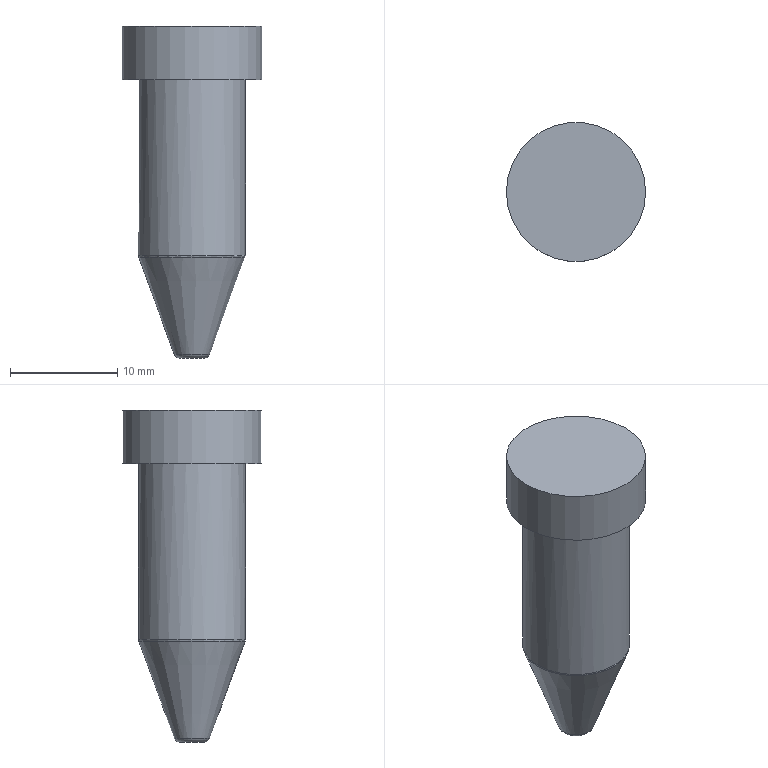Part | STEP file | gslz 2016.10.28-10_id3046_x_t | 1 solid | 8 faces | box 13 x 13 x 31 mm | volume 2308 mm3 | plane 3 | cylinder 2 | torus 2 | cone 1 | commonest cylinder face diameters 10 x1 13 x1
STEP:
#1=CARTESIAN_POINT('',(0.,0.,0.));
#2=DIRECTION('',(0.,0.,1.));
#3=DIRECTION('',(1.,0.,0.));
#4=AXIS2_PLACEMENT_3D('',#1,#2,#3);
#5=CARTESIAN_POINT('',(-528.808,157.,-11.));
#6=VERTEX_POINT('',#5);
#7=CARTESIAN_POINT('',(-531.192,157.,-11.));
#8=VERTEX_POINT('',#7);
#9=CARTESIAN_POINT('',(-530.,157.,-11.));
#10=DIRECTION('',(0.,0.,-1.));
#11=DIRECTION('',(1.,0.,0.));
#12=AXIS2_PLACEMENT_3D('',#9,#10,#11);
#13=CIRCLE('',#12,1.192);
#14=CARTESIAN_POINT('',(-530.,157.,-11.));
#15=DIRECTION('',(0.,0.,1.));
#16=DIRECTION('',(-1.,0.,0.));
#17=AXIS2_PLACEMENT_3D('',#14,#15,#16);
#18=PLANE('',#17);
#19=CARTESIAN_POINT('',(-1.192,0.));
#20=CARTESIAN_POINT('',(-1.192,2.065));
#21=CARTESIAN_POINT('',(0.5961,1.032));
#22=CARTESIAN_POINT('',(2.384,0.));
#23=CARTESIAN_POINT('',(0.5961,-1.032));
#24=CARTESIAN_POINT('',(-1.192,-2.065));
#25=CARTESIAN_POINT('',(-1.192,0.));
#26=(BOUNDED_CURVE()B_SPLINE_CURVE(2,(#19,#20,#21,#22,#23,#24,#25),.UNSPECIFIED.,.T.,.F.)B_SPLINE_CURVE_WITH_KNOTS((1,2,2,2,2,1),(-2.094,0.,2.094,4.189,6.283,8.378),.UNSPECIFIED.)CURVE()GEOMETRIC_REPRESENTATION_ITEM()RATIONAL_B_SPLINE_CURVE((1.,0.5,1.,0.5,1.,0.5,1.))REPRESENTATION_ITEM(''));
#27=(GEOMETRIC_REPRESENTATION_CONTEXT(2)PARAMETRIC_REPRESENTATION_CONTEXT()REPRESENTATION_CONTEXT('',''));
#28=DEFINITIONAL_REPRESENTATION('',(#26),#27);
#29=PCURVE('',#18,#28);
#30=CARTESIAN_POINT('',(-530.,157.,-10.5));
#31=DIRECTION('',(0.,0.,1.));
#32=DIRECTION('',(-1.,0.,0.));
#33=AXIS2_PLACEMENT_3D('',#30,#31,#32);
#34=TOROIDAL_SURFACE('',#33,1.192,0.5);
#35=CARTESIAN_POINT('',(3.142,4.712));
#36=DIRECTION('',(-1.,0.));
#37=VECTOR('',#36,1.);
#38=LINE('',#35,#37);
#39=(GEOMETRIC_REPRESENTATION_CONTEXT(2)PARAMETRIC_REPRESENTATION_CONTEXT()REPRESENTATION_CONTEXT('',''));
#40=DEFINITIONAL_REPRESENTATION('',(#38),#39);
#41=PCURVE('',#34,#40);
#42=SURFACE_CURVE('',#13,(#29,#41),.PCURVE_S1.);
#43=EDGE_CURVE('',#6,#8,#42,.T.);
#44=ORIENTED_EDGE('',*,*,#43,.T.);
#45=CARTESIAN_POINT('',(-530.,157.,-11.));
#46=DIRECTION('',(0.,0.,-1.));
#47=DIRECTION('',(1.,0.,0.));
#48=AXIS2_PLACEMENT_3D('',#45,#46,#47);
#49=CIRCLE('',#48,1.192);
#50=CARTESIAN_POINT('',(-1.192,0.));
#51=CARTESIAN_POINT('',(-1.192,2.065));
#52=CARTESIAN_POINT('',(0.5961,1.032));
#53=CARTESIAN_POINT('',(2.384,0.));
#54=CARTESIAN_POINT('',(0.5961,-1.032));
#55=CARTESIAN_POINT('',(-1.192,-2.065));
#56=CARTESIAN_POINT('',(-1.192,0.));
#57=(BOUNDED_CURVE()B_SPLINE_CURVE(2,(#50,#51,#52,#53,#54,#55,#56),.UNSPECIFIED.,.T.,.F.)B_SPLINE_CURVE_WITH_KNOTS((1,2,2,2,2,1),(-2.094,0.,2.094,4.189,6.283,8.378),.UNSPECIFIED.)CURVE()GEOMETRIC_REPRESENTATION_ITEM()RATIONAL_B_SPLINE_CURVE((1.,0.5,1.,0.5,1.,0.5,1.))REPRESENTATION_ITEM(''));
#58=(GEOMETRIC_REPRESENTATION_CONTEXT(2)PARAMETRIC_REPRESENTATION_CONTEXT()REPRESENTATION_CONTEXT('',''));
#59=DEFINITIONAL_REPRESENTATION('',(#57),#58);
#60=PCURVE('',#18,#59);
#61=CARTESIAN_POINT('',(9.425,4.712));
#62=DIRECTION('',(-1.,0.));
#63=VECTOR('',#62,1.);
#64=LINE('',#61,#63);
#65=(GEOMETRIC_REPRESENTATION_CONTEXT(2)PARAMETRIC_REPRESENTATION_CONTEXT()REPRESENTATION_CONTEXT('',''));
#66=DEFINITIONAL_REPRESENTATION('',(#64),#65);
#67=PCURVE('',#34,#66);
#68=SURFACE_CURVE('',#49,(#60,#67),.PCURVE_S1.);
#69=EDGE_CURVE('',#8,#6,#68,.T.);
#70=ORIENTED_EDGE('',*,*,#69,.T.);
#71=EDGE_LOOP('',(#44,#70));
#72=FACE_BOUND('',#71,.T.);
#73=ADVANCED_FACE('',(#72),#18,.F.);
#74=CARTESIAN_POINT('',(-525.,157.,-1.412));
#75=VERTEX_POINT('',#74);
#76=CARTESIAN_POINT('',(-535.,157.,-1.412));
#77=VERTEX_POINT('',#76);
#78=CARTESIAN_POINT('',(-530.,157.,-1.412));
#79=DIRECTION('',(0.,0.,1.));
#80=DIRECTION('',(1.,0.,0.));
#81=AXIS2_PLACEMENT_3D('',#78,#79,#80);
#82=CIRCLE('',#81,5.);
#83=CARTESIAN_POINT('',(-530.,157.,11.));
#84=DIRECTION('',(0.,0.,-1.));
#85=DIRECTION('',(1.,0.,0.));
#86=AXIS2_PLACEMENT_3D('',#83,#84,#85);
#87=CYLINDRICAL_SURFACE('',#86,5.);
#88=CARTESIAN_POINT('',(6.283,12.412));
#89=DIRECTION('',(-1.,0.));
#90=VECTOR('',#89,1.);
#91=LINE('',#88,#90);
#92=(GEOMETRIC_REPRESENTATION_CONTEXT(2)PARAMETRIC_REPRESENTATION_CONTEXT()REPRESENTATION_CONTEXT('',''));
#93=DEFINITIONAL_REPRESENTATION('',(#91),#92);
#94=PCURVE('',#87,#93);
#95=CARTESIAN_POINT('',(-530.,157.,-1.412));
#96=DIRECTION('',(0.,0.,1.));
#97=DIRECTION('',(-1.,0.,0.));
#98=AXIS2_PLACEMENT_3D('',#95,#96,#97);
#99=TOROIDAL_SURFACE('',#98,4.5,0.5);
#100=CARTESIAN_POINT('',(3.142,6.283));
#101=DIRECTION('',(1.,0.));
#102=VECTOR('',#101,1.);
#103=LINE('',#100,#102);
#104=(GEOMETRIC_REPRESENTATION_CONTEXT(2)PARAMETRIC_REPRESENTATION_CONTEXT()REPRESENTATION_CONTEXT('',''));
#105=DEFINITIONAL_REPRESENTATION('',(#103),#104);
#106=PCURVE('',#99,#105);
#107=SURFACE_CURVE('',#82,(#94,#106),.PCURVE_S1.);
#108=EDGE_CURVE('',#75,#77,#107,.T.);
#109=ORIENTED_EDGE('',*,*,#108,.T.);
#110=CARTESIAN_POINT('',(-530.,157.,-1.412));
#111=DIRECTION('',(0.,0.,1.));
#112=DIRECTION('',(1.,0.,0.));
#113=AXIS2_PLACEMENT_3D('',#110,#111,#112);
#114=CIRCLE('',#113,5.);
#115=CARTESIAN_POINT('',(6.283,12.412));
#116=DIRECTION('',(-1.,0.));
#117=VECTOR('',#116,1.);
#118=LINE('',#115,#117);
#119=(GEOMETRIC_REPRESENTATION_CONTEXT(2)PARAMETRIC_REPRESENTATION_CONTEXT()REPRESENTATION_CONTEXT('',''));
#120=DEFINITIONAL_REPRESENTATION('',(#118),#119);
#121=PCURVE('',#87,#120);
#122=CARTESIAN_POINT('',(-3.142,6.283));
#123=DIRECTION('',(1.,0.));
#124=VECTOR('',#123,1.);
#125=LINE('',#122,#124);
#126=(GEOMETRIC_REPRESENTATION_CONTEXT(2)PARAMETRIC_REPRESENTATION_CONTEXT()REPRESENTATION_CONTEXT('',''));
#127=DEFINITIONAL_REPRESENTATION('',(#125),#126);
#128=PCURVE('',#99,#127);
#129=SURFACE_CURVE('',#114,(#121,#128),.PCURVE_S1.);
#130=EDGE_CURVE('',#77,#75,#129,.T.);
#131=ORIENTED_EDGE('',*,*,#130,.T.);
#132=CARTESIAN_POINT('',(-525.,157.,15.));
#133=VERTEX_POINT('',#132);
#134=CARTESIAN_POINT('',(-525.,157.,15.));
#135=CARTESIAN_POINT('',(-525.,157.,-1.412));
#136=B_SPLINE_CURVE_WITH_KNOTS('',1,(#134,#135),.UNSPECIFIED.,.F.,.F.,(2,2),(-4.,12.412),.PIECEWISE_BEZIER_KNOTS.);
#137=CARTESIAN_POINT('',(0.,0.));
#138=DIRECTION('',(0.,1.));
#139=VECTOR('',#138,1.);
#140=LINE('',#137,#139);
#141=(GEOMETRIC_REPRESENTATION_CONTEXT(2)PARAMETRIC_REPRESENTATION_CONTEXT()REPRESENTATION_CONTEXT('',''));
#142=DEFINITIONAL_REPRESENTATION('',(#140),#141);
#143=PCURVE('',#87,#142);
#144=CARTESIAN_POINT('',(6.283,0.));
#145=DIRECTION('',(0.,1.));
#146=VECTOR('',#145,1.);
#147=LINE('',#144,#146);
#148=(GEOMETRIC_REPRESENTATION_CONTEXT(2)PARAMETRIC_REPRESENTATION_CONTEXT()REPRESENTATION_CONTEXT('',''));
#149=DEFINITIONAL_REPRESENTATION('',(#147),#148);
#150=PCURVE('',#87,#149);
#151=SEAM_CURVE('',#136,(#143,#150),.PCURVE_S1.);
#152=EDGE_CURVE('',#133,#75,#151,.T.);
#153=ORIENTED_EDGE('',*,*,#152,.F.);
#154=CARTESIAN_POINT('',(-530.,157.,15.));
#155=DIRECTION('',(0.,0.,-1.));
#156=DIRECTION('',(1.,0.,0.));
#157=AXIS2_PLACEMENT_3D('',#154,#155,#156);
#158=CIRCLE('',#157,5.);
#159=CARTESIAN_POINT('',(0.,-4.));
#160=DIRECTION('',(1.,0.));
#161=VECTOR('',#160,1.);
#162=LINE('',#159,#161);
#163=(GEOMETRIC_REPRESENTATION_CONTEXT(2)PARAMETRIC_REPRESENTATION_CONTEXT()REPRESENTATION_CONTEXT('',''));
#164=DEFINITIONAL_REPRESENTATION('',(#162),#163);
#165=PCURVE('',#87,#164);
#166=CARTESIAN_POINT('',(-530.,157.,15.));
#167=DIRECTION('',(0.,0.,-1.));
#168=DIRECTION('',(1.,0.,0.));
#169=AXIS2_PLACEMENT_3D('',#166,#167,#168);
#170=PLANE('',#169);
#171=CARTESIAN_POINT('',(0.,0.));
#172=DIRECTION('',(1.,0.));
#173=AXIS2_PLACEMENT_2D('',#171,#172);
#174=CIRCLE('',#173,5.);
#175=(GEOMETRIC_REPRESENTATION_CONTEXT(2)PARAMETRIC_REPRESENTATION_CONTEXT()REPRESENTATION_CONTEXT('',''));
#176=DEFINITIONAL_REPRESENTATION('',(#174),#175);
#177=PCURVE('',#170,#176);
#178=SURFACE_CURVE('',#158,(#165,#177),.PCURVE_S1.);
#179=EDGE_CURVE('',#133,#133,#178,.T.);
#180=ORIENTED_EDGE('',*,*,#179,.T.);
#181=ORIENTED_EDGE('',*,*,#152,.T.);
#182=EDGE_LOOP('',(#109,#131,#153,#180,#181));
#183=FACE_BOUND('',#182,.T.);
#184=ADVANCED_FACE('',(#183),#87,.T.);
#185=CARTESIAN_POINT('',(-523.5,157.,15.));
#186=VERTEX_POINT('',#185);
#187=CARTESIAN_POINT('',(-530.,157.,15.));
#188=DIRECTION('',(0.,0.,1.));
#189=DIRECTION('',(1.,0.,0.));
#190=AXIS2_PLACEMENT_3D('',#187,#188,#189);
#191=CIRCLE('',#190,6.5);
#192=CARTESIAN_POINT('',(6.5,0.));
#193=CARTESIAN_POINT('',(6.5,-11.258));
#194=CARTESIAN_POINT('',(-3.25,-5.629));
#195=CARTESIAN_POINT('',(-13.,0.));
#196=CARTESIAN_POINT('',(-3.25,5.629));
#197=CARTESIAN_POINT('',(6.5,11.258));
#198=CARTESIAN_POINT('',(6.5,0.));
#199=(BOUNDED_CURVE()B_SPLINE_CURVE(2,(#192,#193,#194,#195,#196,#197,#198),.UNSPECIFIED.,.T.,.F.)B_SPLINE_CURVE_WITH_KNOTS((1,2,2,2,2,1),(-2.094,0.,2.094,4.189,6.283,8.378),.UNSPECIFIED.)CURVE()GEOMETRIC_REPRESENTATION_ITEM()RATIONAL_B_SPLINE_CURVE((1.,0.5,1.,0.5,1.,0.5,1.))REPRESENTATION_ITEM(''));
#200=(GEOMETRIC_REPRESENTATION_CONTEXT(2)PARAMETRIC_REPRESENTATION_CONTEXT()REPRESENTATION_CONTEXT('',''));
#201=DEFINITIONAL_REPRESENTATION('',(#199),#200);
#202=PCURVE('',#170,#201);
#203=CARTESIAN_POINT('',(-530.,157.,20.));
#204=DIRECTION('',(0.,0.,-1.));
#205=DIRECTION('',(1.,0.,0.));
#206=AXIS2_PLACEMENT_3D('',#203,#204,#205);
#207=CYLINDRICAL_SURFACE('',#206,6.5);
#208=CARTESIAN_POINT('',(6.283,5.));
#209=DIRECTION('',(-1.,0.));
#210=VECTOR('',#209,1.);
#211=LINE('',#208,#210);
#212=(GEOMETRIC_REPRESENTATION_CONTEXT(2)PARAMETRIC_REPRESENTATION_CONTEXT()REPRESENTATION_CONTEXT('',''));
#213=DEFINITIONAL_REPRESENTATION('',(#211),#212);
#214=PCURVE('',#207,#213);
#215=SURFACE_CURVE('',#191,(#202,#214),.PCURVE_S1.);
#216=EDGE_CURVE('',#186,#186,#215,.T.);
#217=ORIENTED_EDGE('',*,*,#216,.F.);
#218=EDGE_LOOP('',(#217));
#219=FACE_BOUND('',#218,.T.);
#220=ORIENTED_EDGE('',*,*,#179,.F.);
#221=EDGE_LOOP('',(#220));
#222=FACE_BOUND('',#221,.T.);
#223=ADVANCED_FACE('',(#219,#222),#170,.T.);
#224=CARTESIAN_POINT('',(-536.5,157.,20.));
#225=VERTEX_POINT('',#224);
#226=CARTESIAN_POINT('',(-523.5,157.,20.));
#227=VERTEX_POINT('',#226);
#228=CARTESIAN_POINT('',(-530.,157.,20.));
#229=DIRECTION('',(0.,0.,-1.));
#230=DIRECTION('',(-1.,0.,0.));
#231=AXIS2_PLACEMENT_3D('',#228,#229,#230);
#232=CIRCLE('',#231,6.5);
#233=CARTESIAN_POINT('',(-530.,157.,20.));
#234=DIRECTION('',(0.,0.,1.));
#235=DIRECTION('',(-1.,0.,0.));
#236=AXIS2_PLACEMENT_3D('',#233,#234,#235);
#237=PLANE('',#236);
#238=CARTESIAN_POINT('',(6.5,0.));
#239=CARTESIAN_POINT('',(6.5,-11.258));
#240=CARTESIAN_POINT('',(-3.25,-5.629));
#241=CARTESIAN_POINT('',(-13.,0.));
#242=CARTESIAN_POINT('',(-3.25,5.629));
#243=CARTESIAN_POINT('',(6.5,11.258));
#244=CARTESIAN_POINT('',(6.5,0.));
#245=(BOUNDED_CURVE()B_SPLINE_CURVE(2,(#238,#239,#240,#241,#242,#243,#244),.UNSPECIFIED.,.T.,.F.)B_SPLINE_CURVE_WITH_KNOTS((1,2,2,2,2,1),(-2.094,0.,2.094,4.189,6.283,8.378),.UNSPECIFIED.)CURVE()GEOMETRIC_REPRESENTATION_ITEM()RATIONAL_B_SPLINE_CURVE((1.,0.5,1.,0.5,1.,0.5,1.))REPRESENTATION_ITEM(''));
#246=(GEOMETRIC_REPRESENTATION_CONTEXT(2)PARAMETRIC_REPRESENTATION_CONTEXT()REPRESENTATION_CONTEXT('',''));
#247=DEFINITIONAL_REPRESENTATION('',(#245),#246);
#248=PCURVE('',#237,#247);
#249=CARTESIAN_POINT('',(3.142,0.));
#250=DIRECTION('',(1.,0.));
#251=VECTOR('',#250,1.);
#252=LINE('',#249,#251);
#253=(GEOMETRIC_REPRESENTATION_CONTEXT(2)PARAMETRIC_REPRESENTATION_CONTEXT()REPRESENTATION_CONTEXT('',''));
#254=DEFINITIONAL_REPRESENTATION('',(#252),#253);
#255=PCURVE('',#207,#254);
#256=SURFACE_CURVE('',#232,(#248,#255),.PCURVE_S1.);
#257=EDGE_CURVE('',#225,#227,#256,.T.);
#258=ORIENTED_EDGE('',*,*,#257,.F.);
#259=CARTESIAN_POINT('',(-530.,157.,20.));
#260=DIRECTION('',(0.,0.,-1.));
#261=DIRECTION('',(-1.,0.,0.));
#262=AXIS2_PLACEMENT_3D('',#259,#260,#261);
#263=CIRCLE('',#262,6.5);
#264=CARTESIAN_POINT('',(6.5,0.));
#265=CARTESIAN_POINT('',(6.5,-11.258));
#266=CARTESIAN_POINT('',(-3.25,-5.629));
#267=CARTESIAN_POINT('',(-13.,0.));
#268=CARTESIAN_POINT('',(-3.25,5.629));
#269=CARTESIAN_POINT('',(6.5,11.258));
#270=CARTESIAN_POINT('',(6.5,0.));
#271=(BOUNDED_CURVE()B_SPLINE_CURVE(2,(#264,#265,#266,#267,#268,#269,#270),.UNSPECIFIED.,.T.,.F.)B_SPLINE_CURVE_WITH_KNOTS((1,2,2,2,2,1),(-2.094,0.,2.094,4.189,6.283,8.378),.UNSPECIFIED.)CURVE()GEOMETRIC_REPRESENTATION_ITEM()RATIONAL_B_SPLINE_CURVE((1.,0.5,1.,0.5,1.,0.5,1.))REPRESENTATION_ITEM(''));
#272=(GEOMETRIC_REPRESENTATION_CONTEXT(2)PARAMETRIC_REPRESENTATION_CONTEXT()REPRESENTATION_CONTEXT('',''));
#273=DEFINITIONAL_REPRESENTATION('',(#271),#272);
#274=PCURVE('',#237,#273);
#275=CARTESIAN_POINT('',(-3.142,0.));
#276=DIRECTION('',(1.,0.));
#277=VECTOR('',#276,1.);
#278=LINE('',#275,#277);
#279=(GEOMETRIC_REPRESENTATION_CONTEXT(2)PARAMETRIC_REPRESENTATION_CONTEXT()REPRESENTATION_CONTEXT('',''));
#280=DEFINITIONAL_REPRESENTATION('',(#278),#279);
#281=PCURVE('',#207,#280);
#282=SURFACE_CURVE('',#263,(#274,#281),.PCURVE_S1.);
#283=EDGE_CURVE('',#227,#225,#282,.T.);
#284=ORIENTED_EDGE('',*,*,#283,.F.);
#285=EDGE_LOOP('',(#258,#284));
#286=FACE_BOUND('',#285,.T.);
#287=ADVANCED_FACE('',(#286),#237,.T.);
#288=ORIENTED_EDGE('',*,*,#216,.T.);
#289=CARTESIAN_POINT('',(-523.5,157.,20.));
#290=CARTESIAN_POINT('',(-523.5,157.,15.));
#291=B_SPLINE_CURVE_WITH_KNOTS('',1,(#289,#290),.UNSPECIFIED.,.F.,.F.,(2,2),(0.,5.),.PIECEWISE_BEZIER_KNOTS.);
#292=CARTESIAN_POINT('',(0.,0.));
#293=DIRECTION('',(0.,1.));
#294=VECTOR('',#293,1.);
#295=LINE('',#292,#294);
#296=(GEOMETRIC_REPRESENTATION_CONTEXT(2)PARAMETRIC_REPRESENTATION_CONTEXT()REPRESENTATION_CONTEXT('',''));
#297=DEFINITIONAL_REPRESENTATION('',(#295),#296);
#298=PCURVE('',#207,#297);
#299=CARTESIAN_POINT('',(6.283,0.));
#300=DIRECTION('',(0.,1.));
#301=VECTOR('',#300,1.);
#302=LINE('',#299,#301);
#303=(GEOMETRIC_REPRESENTATION_CONTEXT(2)PARAMETRIC_REPRESENTATION_CONTEXT()REPRESENTATION_CONTEXT('',''));
#304=DEFINITIONAL_REPRESENTATION('',(#302),#303);
#305=PCURVE('',#207,#304);
#306=SEAM_CURVE('',#291,(#298,#305),.PCURVE_S1.);
#307=EDGE_CURVE('',#227,#186,#306,.T.);
#308=ORIENTED_EDGE('',*,*,#307,.F.);
#309=ORIENTED_EDGE('',*,*,#283,.T.);
#310=ORIENTED_EDGE('',*,*,#257,.T.);
#311=ORIENTED_EDGE('',*,*,#307,.T.);
#312=EDGE_LOOP('',(#288,#308,#309,#310,#311));
#313=FACE_BOUND('',#312,.T.);
#314=ADVANCED_FACE('',(#313),#207,.T.);
#315=CARTESIAN_POINT('',(-534.97,157.,-1.583));
#316=VERTEX_POINT('',#315);
#317=CARTESIAN_POINT('',(-530.,157.,-1.583));
#318=DIRECTION('',(0.,0.,-1.));
#319=DIRECTION('',(-1.,0.,0.));
#320=AXIS2_PLACEMENT_3D('',#317,#318,#319);
#321=CIRCLE('',#320,4.97);
#322=CARTESIAN_POINT('',(-530.,157.,-1.5));
#323=DIRECTION('',(0.,0.,1.));
#324=DIRECTION('',(-1.,0.,0.));
#325=AXIS2_PLACEMENT_3D('',#322,#323,#324);
#326=CONICAL_SURFACE('',#325,5.,0.3491);
#327=CARTESIAN_POINT('',(6.283,-0.08285));
#328=DIRECTION('',(-1.,0.));
#329=VECTOR('',#328,1.);
#330=LINE('',#327,#329);
#331=(GEOMETRIC_REPRESENTATION_CONTEXT(2)PARAMETRIC_REPRESENTATION_CONTEXT()REPRESENTATION_CONTEXT('',''));
#332=DEFINITIONAL_REPRESENTATION('',(#330),#331);
#333=PCURVE('',#326,#332);
#334=CARTESIAN_POINT('',(6.283,5.934));
#335=DIRECTION('',(-1.,0.));
#336=VECTOR('',#335,1.);
#337=LINE('',#334,#336);
#338=(GEOMETRIC_REPRESENTATION_CONTEXT(2)PARAMETRIC_REPRESENTATION_CONTEXT()REPRESENTATION_CONTEXT('',''));
#339=DEFINITIONAL_REPRESENTATION('',(#337),#338);
#340=PCURVE('',#99,#339);
#341=SURFACE_CURVE('',#321,(#333,#340),.PCURVE_S1.);
#342=EDGE_CURVE('',#316,#316,#341,.T.);
#343=ORIENTED_EDGE('',*,*,#342,.T.);
#344=CARTESIAN_POINT('',(-531.662,157.,-10.671));
#345=VERTEX_POINT('',#344);
#346=CARTESIAN_POINT('',(-531.662,157.,-10.671));
#347=CARTESIAN_POINT('',(-534.97,157.,-1.583));
#348=B_SPLINE_CURVE_WITH_KNOTS('',1,(#346,#347),.UNSPECIFIED.,.F.,.F.,(2,2),(-9.76,-0.08816),.PIECEWISE_BEZIER_KNOTS.);
#349=CARTESIAN_POINT('',(0.,0.));
#350=DIRECTION('',(0.,1.));
#351=VECTOR('',#350,1.);
#352=LINE('',#349,#351);
#353=(GEOMETRIC_REPRESENTATION_CONTEXT(2)PARAMETRIC_REPRESENTATION_CONTEXT()REPRESENTATION_CONTEXT('',''));
#354=DEFINITIONAL_REPRESENTATION('',(#352),#353);
#355=PCURVE('',#326,#354);
#356=CARTESIAN_POINT('',(6.283,0.));
#357=DIRECTION('',(0.,1.));
#358=VECTOR('',#357,1.);
#359=LINE('',#356,#358);
#360=(GEOMETRIC_REPRESENTATION_CONTEXT(2)PARAMETRIC_REPRESENTATION_CONTEXT()REPRESENTATION_CONTEXT('',''));
#361=DEFINITIONAL_REPRESENTATION('',(#359),#360);
#362=PCURVE('',#326,#361);
#363=SEAM_CURVE('',#348,(#355,#362),.PCURVE_S1.);
#364=EDGE_CURVE('',#345,#316,#363,.T.);
#365=ORIENTED_EDGE('',*,*,#364,.F.);
#366=CARTESIAN_POINT('',(-530.,157.,-10.671));
#367=DIRECTION('',(0.,0.,1.));
#368=DIRECTION('',(-1.,0.,0.));
#369=AXIS2_PLACEMENT_3D('',#366,#367,#368);
#370=CIRCLE('',#369,1.662);
#371=CARTESIAN_POINT('',(0.,-9.171));
#372=DIRECTION('',(1.,0.));
#373=VECTOR('',#372,1.);
#374=LINE('',#371,#373);
#375=(GEOMETRIC_REPRESENTATION_CONTEXT(2)PARAMETRIC_REPRESENTATION_CONTEXT()REPRESENTATION_CONTEXT('',''));
#376=DEFINITIONAL_REPRESENTATION('',(#374),#375);
#377=PCURVE('',#326,#376);
#378=CARTESIAN_POINT('',(0.,5.934));
#379=DIRECTION('',(1.,0.));
#380=VECTOR('',#379,1.);
#381=LINE('',#378,#380);
#382=(GEOMETRIC_REPRESENTATION_CONTEXT(2)PARAMETRIC_REPRESENTATION_CONTEXT()REPRESENTATION_CONTEXT('',''));
#383=DEFINITIONAL_REPRESENTATION('',(#381),#382);
#384=PCURVE('',#34,#383);
#385=SURFACE_CURVE('',#370,(#377,#384),.PCURVE_S1.);
#386=EDGE_CURVE('',#345,#345,#385,.T.);
#387=ORIENTED_EDGE('',*,*,#386,.T.);
#388=ORIENTED_EDGE('',*,*,#364,.T.);
#389=EDGE_LOOP('',(#343,#365,#387,#388));
#390=FACE_BOUND('',#389,.T.);
#391=ADVANCED_FACE('',(#390),#326,.T.);
#392=ORIENTED_EDGE('',*,*,#386,.F.);
#393=CARTESIAN_POINT('',(-531.192,157.,-11.));
#394=CARTESIAN_POINT('',(-531.295,157.,-11.));
#395=CARTESIAN_POINT('',(-531.397,157.,-10.975));
#396=CARTESIAN_POINT('',(-531.49,157.,-10.925));
#397=CARTESIAN_POINT('',(-531.568,157.,-10.855));
#398=CARTESIAN_POINT('',(-531.627,157.,-10.768));
#399=CARTESIAN_POINT('',(-531.662,157.,-10.671));
#400=(BOUNDED_CURVE()B_SPLINE_CURVE(6,(#393,#394,#395,#396,#397,#398,#399),.UNSPECIFIED.,.F.,.F.)B_SPLINE_CURVE_WITH_KNOTS((7,7),(4.712,5.934),.PIECEWISE_BEZIER_KNOTS.)CURVE()GEOMETRIC_REPRESENTATION_ITEM()RATIONAL_B_SPLINE_CURVE((1.019,1.006,0.9987,0.9963,0.9987,1.006,1.019))REPRESENTATION_ITEM(''));
#401=CARTESIAN_POINT('',(0.,0.));
#402=DIRECTION('',(0.,1.));
#403=VECTOR('',#402,1.);
#404=LINE('',#401,#403);
#405=(GEOMETRIC_REPRESENTATION_CONTEXT(2)PARAMETRIC_REPRESENTATION_CONTEXT()REPRESENTATION_CONTEXT('',''));
#406=DEFINITIONAL_REPRESENTATION('',(#404),#405);
#407=PCURVE('',#34,#406);
#408=CARTESIAN_POINT('',(6.283,0.));
#409=DIRECTION('',(0.,1.));
#410=VECTOR('',#409,1.);
#411=LINE('',#408,#410);
#412=(GEOMETRIC_REPRESENTATION_CONTEXT(2)PARAMETRIC_REPRESENTATION_CONTEXT()REPRESENTATION_CONTEXT('',''));
#413=DEFINITIONAL_REPRESENTATION('',(#411),#412);
#414=PCURVE('',#34,#413);
#415=SEAM_CURVE('',#400,(#407,#414),.PCURVE_S1.);
#416=EDGE_CURVE('',#8,#345,#415,.T.);
#417=ORIENTED_EDGE('',*,*,#416,.F.);
#418=ORIENTED_EDGE('',*,*,#43,.F.);
#419=ORIENTED_EDGE('',*,*,#69,.F.);
#420=ORIENTED_EDGE('',*,*,#416,.T.);
#421=EDGE_LOOP('',(#392,#417,#418,#419,#420));
#422=FACE_BOUND('',#421,.T.);
#423=ADVANCED_FACE('',(#422),#34,.T.);
#424=ORIENTED_EDGE('',*,*,#342,.F.);
#425=CARTESIAN_POINT('',(-534.97,157.,-1.583));
#426=CARTESIAN_POINT('',(-534.98,157.,-1.555));
#427=CARTESIAN_POINT('',(-534.988,157.,-1.527));
#428=CARTESIAN_POINT('',(-534.994,157.,-1.499));
#429=CARTESIAN_POINT('',(-534.998,157.,-1.47));
#430=CARTESIAN_POINT('',(-535.,157.,-1.441));
#431=CARTESIAN_POINT('',(-535.,157.,-1.412));
#432=(BOUNDED_CURVE()B_SPLINE_CURVE(6,(#425,#426,#427,#428,#429,#430,#431),.UNSPECIFIED.,.F.,.F.)B_SPLINE_CURVE_WITH_KNOTS((7,7),(5.934,6.283),.PIECEWISE_BEZIER_KNOTS.)CURVE()GEOMETRIC_REPRESENTATION_ITEM()RATIONAL_B_SPLINE_CURVE((1.002,1.001,0.9999,0.9997,0.9999,1.001,1.002))REPRESENTATION_ITEM(''));
#433=CARTESIAN_POINT('',(6.283,0.));
#434=DIRECTION('',(0.,1.));
#435=VECTOR('',#434,1.);
#436=LINE('',#433,#435);
#437=(GEOMETRIC_REPRESENTATION_CONTEXT(2)PARAMETRIC_REPRESENTATION_CONTEXT()REPRESENTATION_CONTEXT('',''));
#438=DEFINITIONAL_REPRESENTATION('',(#436),#437);
#439=PCURVE('',#99,#438);
#440=CARTESIAN_POINT('',(0.,0.));
#441=DIRECTION('',(0.,1.));
#442=VECTOR('',#441,1.);
#443=LINE('',#440,#442);
#444=(GEOMETRIC_REPRESENTATION_CONTEXT(2)PARAMETRIC_REPRESENTATION_CONTEXT()REPRESENTATION_CONTEXT('',''));
#445=DEFINITIONAL_REPRESENTATION('',(#443),#444);
#446=PCURVE('',#99,#445);
#447=SEAM_CURVE('',#432,(#439,#446),.PCURVE_S1.);
#448=EDGE_CURVE('',#316,#77,#447,.T.);
#449=ORIENTED_EDGE('',*,*,#448,.T.);
#450=ORIENTED_EDGE('',*,*,#108,.F.);
#451=ORIENTED_EDGE('',*,*,#130,.F.);
#452=ORIENTED_EDGE('',*,*,#448,.F.);
#453=EDGE_LOOP('',(#424,#449,#450,#451,#452));
#454=FACE_BOUND('',#453,.T.);
#455=ADVANCED_FACE('',(#454),#99,.T.);
#456=CLOSED_SHELL('',(#73,#184,#223,#287,#314,#391,#423,#455));
#457=MANIFOLD_SOLID_BREP('',#456);
#458=(LENGTH_UNIT()NAMED_UNIT(*)SI_UNIT(.MILLI.,.METRE.));
#459=UNCERTAINTY_MEASURE_WITH_UNIT(LENGTH_MEASURE(0.000005),#458,'','');
#460=(NAMED_UNIT(*)PLANE_ANGLE_UNIT()SI_UNIT($,.RADIAN.));
#461=(NAMED_UNIT(*)SI_UNIT($,.STERADIAN.)SOLID_ANGLE_UNIT());
#462=(GEOMETRIC_REPRESENTATION_CONTEXT(3)GLOBAL_UNCERTAINTY_ASSIGNED_CONTEXT((#459))GLOBAL_UNIT_ASSIGNED_CONTEXT((#458,#460,#461))REPRESENTATION_CONTEXT('',''));
#463=ADVANCED_BREP_SHAPE_REPRESENTATION('',(#4,#457),#462);